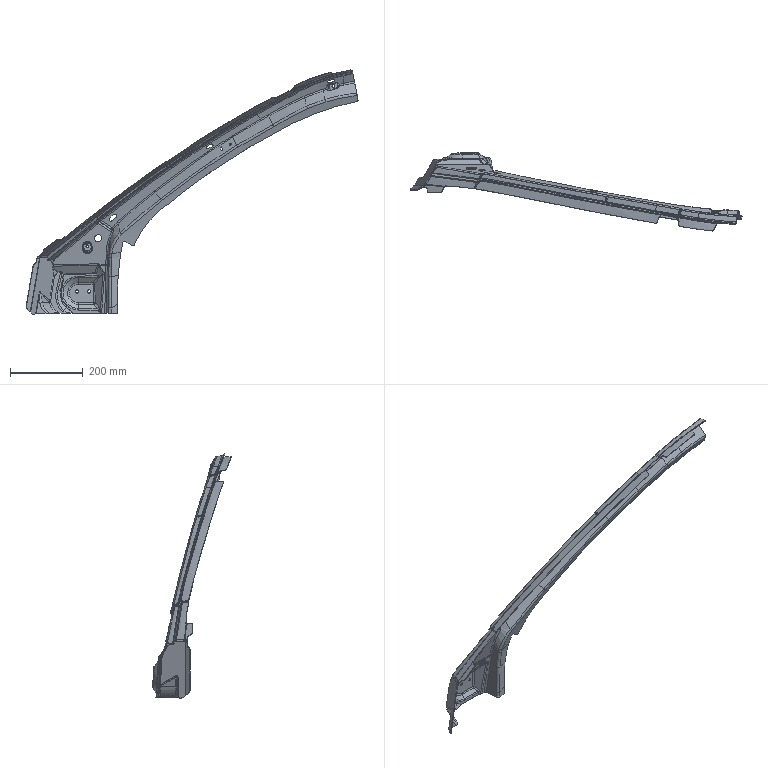Part | STEP file | FNA5401212 | 1 solid | 670 faces | box 914.927 x 216.551 x 677.274 mm | volume 214602 mm3 | spline 542 | cylinder 82 | plane 27 | sphere 14 | other 5 | commonest cylinder face diameters 12 x16 9.6 x12 16 x7 10 x6 13.6 x5 20 x5